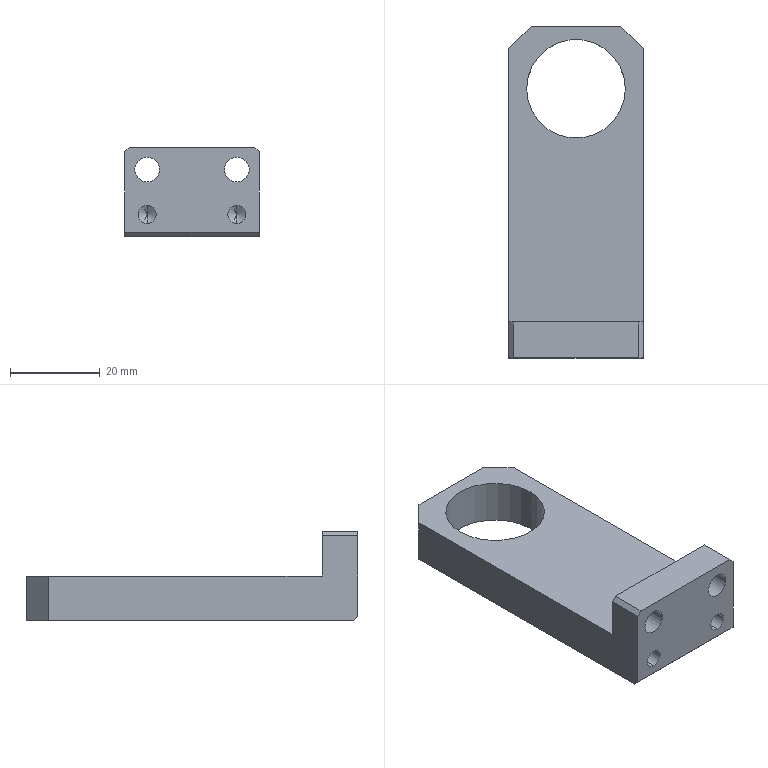Part | SolidWorks | features Chamfer 2, ICE 2, Extrusion 1, HoleWzd 1 | 1 solid | 27 faces | box 30 x 74 x 20 mm | volume 19884 mm3 | plane 13 | cylinder 10 | cone 4 | commonest cylinder face diameters 4 x4 5.5 x4 22 x2
STEP:
#1=CARTESIAN_POINT('',(-10.,10.,7.));
#2=VERTEX_POINT('',#1);
#3=CARTESIAN_POINT('',(-10.,10.,3.));
#4=VERTEX_POINT('',#3);
#5=CARTESIAN_POINT('',(-10.,10.,5.));
#6=DIRECTION('',(0.,-1.,0.));
#7=DIRECTION('',(0.,0.,-1.));
#8=AXIS2_PLACEMENT_3D('',#5,#6,#7);
#9=CIRCLE('',#8,2.);
#10=EDGE_CURVE('',#2,#4,#9,.T.);
#11=ORIENTED_EDGE('',*,*,#10,.F.);
#12=CARTESIAN_POINT('',(-10.,0.,7.));
#13=VERTEX_POINT('',#12);
#14=CARTESIAN_POINT('',(-10.,0.,7.));
#15=DIRECTION('',(0.,-1.,0.));
#16=VECTOR('',#15,1000.);
#17=LINE('',#14,#16);
#18=EDGE_CURVE('',#2,#13,#17,.T.);
#19=ORIENTED_EDGE('',*,*,#18,.T.);
#20=CARTESIAN_POINT('',(-10.,0.,3.));
#21=VERTEX_POINT('',#20);
#22=CARTESIAN_POINT('',(-10.,0.,5.));
#23=DIRECTION('',(0.,-1.,0.));
#24=DIRECTION('',(0.,0.,-1.));
#25=AXIS2_PLACEMENT_3D('',#22,#23,#24);
#26=CIRCLE('',#25,2.);
#27=EDGE_CURVE('',#13,#21,#26,.T.);
#28=ORIENTED_EDGE('',*,*,#27,.T.);
#29=CARTESIAN_POINT('',(-10.,0.,3.));
#30=DIRECTION('',(0.,-1.,0.));
#31=VECTOR('',#30,1000.);
#32=LINE('',#29,#31);
#33=EDGE_CURVE('',#4,#21,#32,.T.);
#34=ORIENTED_EDGE('',*,*,#33,.F.);
#35=EDGE_LOOP('',(#11,#19,#28,#34));
#36=FACE_OUTER_BOUND('',#35,.T.);
#37=CARTESIAN_POINT('',(-10.,0.,5.));
#38=DIRECTION('',(0.,-1.,0.));
#39=DIRECTION('',(0.,0.,-1.));
#40=AXIS2_PLACEMENT_3D('',#37,#38,#39);
#41=CYLINDRICAL_SURFACE('',#40,2.);
#42=ADVANCED_FACE('',(#36),#41,.F.);
#43=CARTESIAN_POINT('',(-10.,11.202,5.));
#44=VERTEX_POINT('',#43);
#45=CARTESIAN_POINT('',(-10.,10.,3.));
#46=DIRECTION('',(0.,-0.515,-0.8572));
#47=VECTOR('',#46,1000.);
#48=LINE('',#45,#47);
#49=EDGE_CURVE('',#44,#4,#48,.T.);
#50=ORIENTED_EDGE('',*,*,#49,.F.);
#51=CARTESIAN_POINT('',(-10.,10.,7.));
#52=DIRECTION('',(0.,-0.515,0.8572));
#53=VECTOR('',#52,1000.);
#54=LINE('',#51,#53);
#55=EDGE_CURVE('',#44,#2,#54,.T.);
#56=ORIENTED_EDGE('',*,*,#55,.T.);
#57=ORIENTED_EDGE('',*,*,#10,.T.);
#58=EDGE_LOOP('',(#50,#56,#57));
#59=FACE_OUTER_BOUND('',#58,.T.);
#60=CARTESIAN_POINT('',(-10.,10.,5.));
#61=DIRECTION('',(0.,-1.,0.));
#62=DIRECTION('',(0.,0.,-1.));
#63=AXIS2_PLACEMENT_3D('',#60,#61,#62);
#64=CONICAL_SURFACE('',#63,2.,1.03);
#65=ADVANCED_FACE('',(#59),#64,.F.);
#66=CARTESIAN_POINT('',(10.,10.,7.));
#67=VERTEX_POINT('',#66);
#68=CARTESIAN_POINT('',(10.,10.,3.));
#69=VERTEX_POINT('',#68);
#70=CARTESIAN_POINT('',(10.,10.,5.));
#71=DIRECTION('',(0.,-1.,0.));
#72=DIRECTION('',(0.,0.,-1.));
#73=AXIS2_PLACEMENT_3D('',#70,#71,#72);
#74=CIRCLE('',#73,2.);
#75=EDGE_CURVE('',#67,#69,#74,.T.);
#76=ORIENTED_EDGE('',*,*,#75,.F.);
#77=CARTESIAN_POINT('',(10.,0.,7.));
#78=VERTEX_POINT('',#77);
#79=CARTESIAN_POINT('',(10.,0.,7.));
#80=DIRECTION('',(0.,-1.,0.));
#81=VECTOR('',#80,1000.);
#82=LINE('',#79,#81);
#83=EDGE_CURVE('',#67,#78,#82,.T.);
#84=ORIENTED_EDGE('',*,*,#83,.T.);
#85=CARTESIAN_POINT('',(10.,0.,3.));
#86=VERTEX_POINT('',#85);
#87=CARTESIAN_POINT('',(10.,0.,5.));
#88=DIRECTION('',(0.,-1.,0.));
#89=DIRECTION('',(0.,0.,-1.));
#90=AXIS2_PLACEMENT_3D('',#87,#88,#89);
#91=CIRCLE('',#90,2.);
#92=EDGE_CURVE('',#78,#86,#91,.T.);
#93=ORIENTED_EDGE('',*,*,#92,.T.);
#94=CARTESIAN_POINT('',(10.,0.,3.));
#95=DIRECTION('',(0.,-1.,0.));
#96=VECTOR('',#95,1000.);
#97=LINE('',#94,#96);
#98=EDGE_CURVE('',#69,#86,#97,.T.);
#99=ORIENTED_EDGE('',*,*,#98,.F.);
#100=EDGE_LOOP('',(#76,#84,#93,#99));
#101=FACE_OUTER_BOUND('',#100,.T.);
#102=CARTESIAN_POINT('',(10.,0.,5.));
#103=DIRECTION('',(0.,-1.,0.));
#104=DIRECTION('',(0.,0.,-1.));
#105=AXIS2_PLACEMENT_3D('',#102,#103,#104);
#106=CYLINDRICAL_SURFACE('',#105,2.);
#107=ADVANCED_FACE('',(#101),#106,.F.);
#108=CARTESIAN_POINT('',(10.,11.202,5.));
#109=VERTEX_POINT('',#108);
#110=CARTESIAN_POINT('',(10.,10.,3.));
#111=DIRECTION('',(0.,-0.515,-0.8572));
#112=VECTOR('',#111,1000.);
#113=LINE('',#110,#112);
#114=EDGE_CURVE('',#109,#69,#113,.T.);
#115=ORIENTED_EDGE('',*,*,#114,.F.);
#116=CARTESIAN_POINT('',(10.,10.,7.));
#117=DIRECTION('',(0.,-0.515,0.8572));
#118=VECTOR('',#117,1000.);
#119=LINE('',#116,#118);
#120=EDGE_CURVE('',#109,#67,#119,.T.);
#121=ORIENTED_EDGE('',*,*,#120,.T.);
#122=ORIENTED_EDGE('',*,*,#75,.T.);
#123=EDGE_LOOP('',(#115,#121,#122));
#124=FACE_OUTER_BOUND('',#123,.T.);
#125=CARTESIAN_POINT('',(10.,10.,5.));
#126=DIRECTION('',(0.,-1.,0.));
#127=DIRECTION('',(0.,0.,-1.));
#128=AXIS2_PLACEMENT_3D('',#125,#126,#127);
#129=CONICAL_SURFACE('',#128,2.,1.03);
#130=ADVANCED_FACE('',(#124),#129,.F.);
#131=CARTESIAN_POINT('',(12.75,0.,15.));
#132=VERTEX_POINT('',#131);
#133=CARTESIAN_POINT('',(7.25,0.,15.));
#134=VERTEX_POINT('',#133);
#135=CARTESIAN_POINT('',(10.,0.,15.));
#136=DIRECTION('',(0.,1.,0.));
#137=DIRECTION('',(1.,0.,0.));
#138=AXIS2_PLACEMENT_3D('',#135,#136,#137);
#139=CIRCLE('',#138,2.75);
#140=EDGE_CURVE('',#132,#134,#139,.T.);
#141=ORIENTED_EDGE('',*,*,#140,.F.);
#142=CARTESIAN_POINT('',(12.75,8.,15.));
#143=VERTEX_POINT('',#142);
#144=CARTESIAN_POINT('',(12.75,0.,15.));
#145=DIRECTION('',(0.,1.,0.));
#146=VECTOR('',#145,1000.);
#147=LINE('',#144,#146);
#148=EDGE_CURVE('',#132,#143,#147,.T.);
#149=ORIENTED_EDGE('',*,*,#148,.T.);
#150=CARTESIAN_POINT('',(7.25,8.,15.));
#151=VERTEX_POINT('',#150);
#152=CARTESIAN_POINT('',(10.,8.,15.));
#153=DIRECTION('',(0.,1.,0.));
#154=DIRECTION('',(1.,0.,0.));
#155=AXIS2_PLACEMENT_3D('',#152,#153,#154);
#156=CIRCLE('',#155,2.75);
#157=EDGE_CURVE('',#143,#151,#156,.T.);
#158=ORIENTED_EDGE('',*,*,#157,.T.);
#159=CARTESIAN_POINT('',(7.25,0.,15.));
#160=DIRECTION('',(0.,1.,0.));
#161=VECTOR('',#160,1000.);
#162=LINE('',#159,#161);
#163=EDGE_CURVE('',#134,#151,#162,.T.);
#164=ORIENTED_EDGE('',*,*,#163,.F.);
#165=EDGE_LOOP('',(#141,#149,#158,#164));
#166=FACE_OUTER_BOUND('',#165,.T.);
#167=CARTESIAN_POINT('',(10.,0.,15.));
#168=DIRECTION('',(0.,1.,0.));
#169=DIRECTION('',(-1.,0.,0.));
#170=AXIS2_PLACEMENT_3D('',#167,#168,#169);
#171=CYLINDRICAL_SURFACE('',#170,2.75);
#172=ADVANCED_FACE('',(#166),#171,.F.);
#173=CARTESIAN_POINT('',(-7.25,0.,15.));
#174=VERTEX_POINT('',#173);
#175=CARTESIAN_POINT('',(-12.75,0.,15.));
#176=VERTEX_POINT('',#175);
#177=CARTESIAN_POINT('',(-10.,0.,15.));
#178=DIRECTION('',(0.,1.,0.));
#179=DIRECTION('',(-1.,0.,0.));
#180=AXIS2_PLACEMENT_3D('',#177,#178,#179);
#181=CIRCLE('',#180,2.75);
#182=EDGE_CURVE('',#174,#176,#181,.T.);
#183=ORIENTED_EDGE('',*,*,#182,.F.);
#184=CARTESIAN_POINT('',(-7.25,8.,15.));
#185=VERTEX_POINT('',#184);
#186=CARTESIAN_POINT('',(-7.25,0.,15.));
#187=DIRECTION('',(0.,1.,0.));
#188=VECTOR('',#187,1000.);
#189=LINE('',#186,#188);
#190=EDGE_CURVE('',#174,#185,#189,.T.);
#191=ORIENTED_EDGE('',*,*,#190,.T.);
#192=CARTESIAN_POINT('',(-12.75,8.,15.));
#193=VERTEX_POINT('',#192);
#194=CARTESIAN_POINT('',(-10.,8.,15.));
#195=DIRECTION('',(0.,1.,0.));
#196=DIRECTION('',(-1.,0.,0.));
#197=AXIS2_PLACEMENT_3D('',#194,#195,#196);
#198=CIRCLE('',#197,2.75);
#199=EDGE_CURVE('',#185,#193,#198,.T.);
#200=ORIENTED_EDGE('',*,*,#199,.T.);
#201=CARTESIAN_POINT('',(-12.75,0.,15.));
#202=DIRECTION('',(0.,1.,0.));
#203=VECTOR('',#202,1000.);
#204=LINE('',#201,#203);
#205=EDGE_CURVE('',#176,#193,#204,.T.);
#206=ORIENTED_EDGE('',*,*,#205,.F.);
#207=EDGE_LOOP('',(#183,#191,#200,#206));
#208=FACE_OUTER_BOUND('',#207,.T.);
#209=CARTESIAN_POINT('',(-10.,0.,15.));
#210=DIRECTION('',(0.,1.,0.));
#211=DIRECTION('',(-1.,0.,0.));
#212=AXIS2_PLACEMENT_3D('',#209,#210,#211);
#213=CYLINDRICAL_SURFACE('',#212,2.75);
#214=ADVANCED_FACE('',(#208),#213,.F.);
#215=CARTESIAN_POINT('',(-11.,60.,10.));
#216=VERTEX_POINT('',#215);
#217=CARTESIAN_POINT('',(11.,60.,10.));
#218=VERTEX_POINT('',#217);
#219=CARTESIAN_POINT('',(0.,60.,10.));
#220=DIRECTION('',(0.,0.,1.));
#221=DIRECTION('',(1.,0.,0.));
#222=AXIS2_PLACEMENT_3D('',#219,#220,#221);
#223=CIRCLE('',#222,11.);
#224=EDGE_CURVE('',#216,#218,#223,.T.);
#225=ORIENTED_EDGE('',*,*,#224,.T.);
#226=CARTESIAN_POINT('',(11.,60.,0.));
#227=VERTEX_POINT('',#226);
#228=CARTESIAN_POINT('',(11.,60.,10.));
#229=DIRECTION('',(0.,0.,-1.));
#230=VECTOR('',#229,1000.);
#231=LINE('',#228,#230);
#232=EDGE_CURVE('',#218,#227,#231,.T.);
#233=ORIENTED_EDGE('',*,*,#232,.T.);
#234=CARTESIAN_POINT('',(-11.,60.,0.));
#235=VERTEX_POINT('',#234);
#236=CARTESIAN_POINT('',(0.,60.,0.));
#237=DIRECTION('',(0.,0.,1.));
#238=DIRECTION('',(1.,0.,0.));
#239=AXIS2_PLACEMENT_3D('',#236,#237,#238);
#240=CIRCLE('',#239,11.);
#241=EDGE_CURVE('',#235,#227,#240,.T.);
#242=ORIENTED_EDGE('',*,*,#241,.F.);
#243=CARTESIAN_POINT('',(-11.,60.,10.));
#244=DIRECTION('',(0.,0.,-1.));
#245=VECTOR('',#244,1000.);
#246=LINE('',#243,#245);
#247=EDGE_CURVE('',#216,#235,#246,.T.);
#248=ORIENTED_EDGE('',*,*,#247,.F.);
#249=EDGE_LOOP('',(#225,#233,#242,#248));
#250=FACE_OUTER_BOUND('',#249,.T.);
#251=CARTESIAN_POINT('',(0.,60.,10.));
#252=DIRECTION('',(0.,0.,-1.));
#253=DIRECTION('',(-1.,0.,0.));
#254=AXIS2_PLACEMENT_3D('',#251,#252,#253);
#255=CYLINDRICAL_SURFACE('',#254,11.);
#256=ADVANCED_FACE('',(#250),#255,.F.);
#257=CARTESIAN_POINT('',(10.,74.,10.));
#258=VERTEX_POINT('',#257);
#259=CARTESIAN_POINT('',(-10.,74.,10.));
#260=VERTEX_POINT('',#259);
#261=CARTESIAN_POINT('',(15.,74.,10.));
#262=DIRECTION('',(-1.,0.,0.));
#263=VECTOR('',#262,1000.);
#264=LINE('',#261,#263);
#265=EDGE_CURVE('',#258,#260,#264,.T.);
#266=ORIENTED_EDGE('',*,*,#265,.T.);
#267=CARTESIAN_POINT('',(-15.,69.,10.));
#268=VERTEX_POINT('',#267);
#269=CARTESIAN_POINT('',(-12.5,71.5,10.));
#270=DIRECTION('',(-0.7071,-0.7071,0.));
#271=VECTOR('',#270,1000.);
#272=LINE('',#269,#271);
#273=EDGE_CURVE('',#260,#268,#272,.T.);
#274=ORIENTED_EDGE('',*,*,#273,.T.);
#275=CARTESIAN_POINT('',(-15.,8.,10.));
#276=VERTEX_POINT('',#275);
#277=CARTESIAN_POINT('',(-15.,0.,10.));
#278=DIRECTION('',(0.,-1.,0.));
#279=VECTOR('',#278,1000.);
#280=LINE('',#277,#279);
#281=EDGE_CURVE('',#268,#276,#280,.T.);
#282=ORIENTED_EDGE('',*,*,#281,.T.);
#283=CARTESIAN_POINT('',(15.,8.,10.));
#284=VERTEX_POINT('',#283);
#285=CARTESIAN_POINT('',(0.,8.,10.));
#286=DIRECTION('',(-1.,0.,0.));
#287=VECTOR('',#286,1000.);
#288=LINE('',#285,#287);
#289=EDGE_CURVE('',#284,#276,#288,.T.);
#290=ORIENTED_EDGE('',*,*,#289,.F.);
#291=CARTESIAN_POINT('',(15.,69.,10.));
#292=VERTEX_POINT('',#291);
#293=CARTESIAN_POINT('',(15.,0.,10.));
#294=DIRECTION('',(0.,1.,0.));
#295=VECTOR('',#294,1000.);
#296=LINE('',#293,#295);
#297=EDGE_CURVE('',#284,#292,#296,.T.);
#298=ORIENTED_EDGE('',*,*,#297,.T.);
#299=CARTESIAN_POINT('',(-2.5,86.5,10.));
#300=DIRECTION('',(-0.7071,0.7071,0.));
#301=VECTOR('',#300,1000.);
#302=LINE('',#299,#301);
#303=EDGE_CURVE('',#292,#258,#302,.T.);
#304=ORIENTED_EDGE('',*,*,#303,.T.);
#305=EDGE_LOOP('',(#266,#274,#282,#290,#298,#304));
#306=FACE_OUTER_BOUND('',#305,.T.);
#307=ORIENTED_EDGE('',*,*,#224,.F.);
#308=CARTESIAN_POINT('',(0.,60.,10.));
#309=DIRECTION('',(0.,0.,1.));
#310=DIRECTION('',(1.,0.,0.));
#311=AXIS2_PLACEMENT_3D('',#308,#309,#310);
#312=CIRCLE('',#311,11.);
#313=EDGE_CURVE('',#218,#216,#312,.T.);
#314=ORIENTED_EDGE('',*,*,#313,.F.);
#315=EDGE_LOOP('',(#307,#314));
#316=FACE_BOUND('',#315,.T.);
#317=CARTESIAN_POINT('',(-15.,74.,10.));
#318=DIRECTION('',(0.,0.,1.));
#319=DIRECTION('',(1.,0.,0.));
#320=AXIS2_PLACEMENT_3D('',#317,#318,#319);
#321=PLANE('',#320);
#322=ADVANCED_FACE('',(#306,#316),#321,.T.);
#323=CARTESIAN_POINT('',(15.,1.,0.));
#324=VERTEX_POINT('',#323);
#325=CARTESIAN_POINT('',(15.,69.,0.));
#326=VERTEX_POINT('',#325);
#327=CARTESIAN_POINT('',(15.,0.,0.));
#328=DIRECTION('',(0.,1.,0.));
#329=VECTOR('',#328,1000.);
#330=LINE('',#327,#329);
#331=EDGE_CURVE('',#324,#326,#330,.T.);
#332=ORIENTED_EDGE('',*,*,#331,.F.);
#333=CARTESIAN_POINT('',(-15.,1.,0.));
#334=VERTEX_POINT('',#333);
#335=CARTESIAN_POINT('',(-15.,1.,0.));
#336=DIRECTION('',(-1.,0.,0.));
#337=VECTOR('',#336,1000.);
#338=LINE('',#335,#337);
#339=EDGE_CURVE('',#324,#334,#338,.T.);
#340=ORIENTED_EDGE('',*,*,#339,.T.);
#341=CARTESIAN_POINT('',(-15.,69.,0.));
#342=VERTEX_POINT('',#341);
#343=CARTESIAN_POINT('',(-15.,0.,0.));
#344=DIRECTION('',(0.,-1.,0.));
#345=VECTOR('',#344,1000.);
#346=LINE('',#343,#345);
#347=EDGE_CURVE('',#342,#334,#346,.T.);
#348=ORIENTED_EDGE('',*,*,#347,.F.);
#349=CARTESIAN_POINT('',(-10.,74.,0.));
#350=VERTEX_POINT('',#349);
#351=CARTESIAN_POINT('',(-15.,69.,0.));
#352=DIRECTION('',(0.7071,0.7071,0.));
#353=VECTOR('',#352,1000.);
#354=LINE('',#351,#353);
#355=EDGE_CURVE('',#342,#350,#354,.T.);
#356=ORIENTED_EDGE('',*,*,#355,.T.);
#357=CARTESIAN_POINT('',(10.,74.,0.));
#358=VERTEX_POINT('',#357);
#359=CARTESIAN_POINT('',(15.,74.,0.));
#360=DIRECTION('',(-1.,0.,0.));
#361=VECTOR('',#360,1000.);
#362=LINE('',#359,#361);
#363=EDGE_CURVE('',#358,#350,#362,.T.);
#364=ORIENTED_EDGE('',*,*,#363,.F.);
#365=CARTESIAN_POINT('',(10.,74.,0.));
#366=DIRECTION('',(0.7071,-0.7071,0.));
#367=VECTOR('',#366,1000.);
#368=LINE('',#365,#367);
#369=EDGE_CURVE('',#358,#326,#368,.T.);
#370=ORIENTED_EDGE('',*,*,#369,.T.);
#371=EDGE_LOOP('',(#332,#340,#348,#356,#364,#370));
#372=FACE_OUTER_BOUND('',#371,.T.);
#373=ORIENTED_EDGE('',*,*,#241,.T.);
#374=CARTESIAN_POINT('',(0.,60.,0.));
#375=DIRECTION('',(0.,0.,1.));
#376=DIRECTION('',(1.,0.,0.));
#377=AXIS2_PLACEMENT_3D('',#374,#375,#376);
#378=CIRCLE('',#377,11.);
#379=EDGE_CURVE('',#227,#235,#378,.T.);
#380=ORIENTED_EDGE('',*,*,#379,.T.);
#381=EDGE_LOOP('',(#373,#380));
#382=FACE_BOUND('',#381,.T.);
#383=CARTESIAN_POINT('',(-15.,74.,0.));
#384=DIRECTION('',(0.,0.,1.));
#385=DIRECTION('',(1.,0.,0.));
#386=AXIS2_PLACEMENT_3D('',#383,#384,#385);
#387=PLANE('',#386);
#388=ADVANCED_FACE('',(#372,#382),#387,.F.);
#389=ORIENTED_EDGE('',*,*,#347,.T.);
#390=CARTESIAN_POINT('',(-15.,0.,1.));
#391=VERTEX_POINT('',#390);
#392=CARTESIAN_POINT('',(-15.,0.,1.));
#393=DIRECTION('',(0.,-0.7071,0.7071));
#394=VECTOR('',#393,1000.);
#395=LINE('',#392,#394);
#396=EDGE_CURVE('',#334,#391,#395,.T.);
#397=ORIENTED_EDGE('',*,*,#396,.T.);
#398=CARTESIAN_POINT('',(-15.,0.,19.));
#399=VERTEX_POINT('',#398);
#400=CARTESIAN_POINT('',(-15.,0.,10.));
#401=DIRECTION('',(0.,0.,-1.));
#402=VECTOR('',#401,1000.);
#403=LINE('',#400,#402);
#404=EDGE_CURVE('',#399,#391,#403,.T.);
#405=ORIENTED_EDGE('',*,*,#404,.F.);
#406=CARTESIAN_POINT('',(-15.,8.,19.));
#407=VERTEX_POINT('',#406);
#408=CARTESIAN_POINT('',(-15.,0.,19.));
#409=DIRECTION('',(0.,1.,0.));
#410=VECTOR('',#409,1000.);
#411=LINE('',#408,#410);
#412=EDGE_CURVE('',#399,#407,#411,.T.);
#413=ORIENTED_EDGE('',*,*,#412,.T.);
#414=CARTESIAN_POINT('',(-15.,8.,0.));
#415=DIRECTION('',(0.,0.,1.));
#416=VECTOR('',#415,1000.);
#417=LINE('',#414,#416);
#418=EDGE_CURVE('',#276,#407,#417,.T.);
#419=ORIENTED_EDGE('',*,*,#418,.F.);
#420=ORIENTED_EDGE('',*,*,#281,.F.);
#421=CARTESIAN_POINT('',(-15.,69.,10.));
#422=DIRECTION('',(0.,0.,-1.));
#423=VECTOR('',#422,1000.);
#424=LINE('',#421,#423);
#425=EDGE_CURVE('',#268,#342,#424,.T.);
#426=ORIENTED_EDGE('',*,*,#425,.T.);
#427=EDGE_LOOP('',(#389,#397,#405,#413,#419,#420,#426));
#428=FACE_OUTER_BOUND('',#427,.T.);
#429=CARTESIAN_POINT('',(-15.,0.,10.));
#430=DIRECTION('',(1.,0.,0.));
#431=DIRECTION('',(0.,0.,-1.));
#432=AXIS2_PLACEMENT_3D('',#429,#430,#431);
#433=PLANE('',#432);
#434=ADVANCED_FACE('',(#428),#433,.F.);
#435=CARTESIAN_POINT('',(-10.,0.,5.));
#436=DIRECTION('',(0.,-1.,0.));
#437=DIRECTION('',(0.,0.,-1.));
#438=AXIS2_PLACEMENT_3D('',#435,#436,#437);
#439=CIRCLE('',#438,2.);
#440=EDGE_CURVE('',#21,#13,#439,.T.);
#441=ORIENTED_EDGE('',*,*,#440,.F.);
#442=ORIENTED_EDGE('',*,*,#27,.F.);
#443=EDGE_LOOP('',(#441,#442));
#444=FACE_BOUND('',#443,.T.);
#445=CARTESIAN_POINT('',(10.,0.,5.));
#446=DIRECTION('',(0.,-1.,0.));
#447=DIRECTION('',(0.,0.,-1.));
#448=AXIS2_PLACEMENT_3D('',#445,#446,#447);
#449=CIRCLE('',#448,2.);
#450=EDGE_CURVE('',#86,#78,#449,.T.);
#451=ORIENTED_EDGE('',*,*,#450,.F.);
#452=ORIENTED_EDGE('',*,*,#92,.F.);
#453=EDGE_LOOP('',(#451,#452));
#454=FACE_BOUND('',#453,.T.);
#455=CARTESIAN_POINT('',(10.,0.,15.));
#456=DIRECTION('',(0.,1.,0.));
#457=DIRECTION('',(1.,0.,0.));
#458=AXIS2_PLACEMENT_3D('',#455,#456,#457);
#459=CIRCLE('',#458,2.75);
#460=EDGE_CURVE('',#134,#132,#459,.T.);
#461=ORIENTED_EDGE('',*,*,#460,.T.);
#462=ORIENTED_EDGE('',*,*,#140,.T.);
#463=EDGE_LOOP('',(#461,#462));
#464=FACE_BOUND('',#463,.T.);
#465=CARTESIAN_POINT('',(-10.,0.,15.));
#466=DIRECTION('',(0.,1.,0.));
#467=DIRECTION('',(-1.,0.,0.));
#468=AXIS2_PLACEMENT_3D('',#465,#466,#467);
#469=CIRCLE('',#468,2.75);
#470=EDGE_CURVE('',#176,#174,#469,.T.);
#471=ORIENTED_EDGE('',*,*,#470,.T.);
#472=ORIENTED_EDGE('',*,*,#182,.T.);
#473=EDGE_LOOP('',(#471,#472));
#474=FACE_BOUND('',#473,.T.);
#475=ORIENTED_EDGE('',*,*,#404,.T.);
#476=CARTESIAN_POINT('',(15.,0.,1.));
#477=VERTEX_POINT('',#476);
#478=CARTESIAN_POINT('',(15.,0.,1.));
#479=DIRECTION('',(1.,0.,0.));
#480=VECTOR('',#479,1000.);
#481=LINE('',#478,#480);
#482=EDGE_CURVE('',#391,#477,#481,.T.);
#483=ORIENTED_EDGE('',*,*,#482,.T.);
#484=CARTESIAN_POINT('',(15.,0.,19.));
#485=VERTEX_POINT('',#484);
#486=CARTESIAN_POINT('',(15.,0.,10.));
#487=DIRECTION('',(0.,0.,-1.));
#488=VECTOR('',#487,1000.);
#489=LINE('',#486,#488);
#490=EDGE_CURVE('',#485,#477,#489,.T.);
#491=ORIENTED_EDGE('',*,*,#490,.F.);
#492=CARTESIAN_POINT('',(14.,0.,20.));
#493=VERTEX_POINT('',#492);
#494=CARTESIAN_POINT('',(15.,0.,19.));
#495=DIRECTION('',(-0.7071,0.,0.7071));
#496=VECTOR('',#495,1000.);
#497=LINE('',#494,#496);
#498=EDGE_CURVE('',#485,#493,#497,.T.);
#499=ORIENTED_EDGE('',*,*,#498,.T.);
#500=CARTESIAN_POINT('',(-14.,0.,20.));
#501=VERTEX_POINT('',#500);
#502=CARTESIAN_POINT('',(0.,0.,20.));
#503=DIRECTION('',(1.,0.,0.));
#504=VECTOR('',#503,1000.);
#505=LINE('',#502,#504);
#506=EDGE_CURVE('',#501,#493,#505,.T.);
#507=ORIENTED_EDGE('',*,*,#506,.F.);
#508=CARTESIAN_POINT('',(-14.,0.,20.));
#509=DIRECTION('',(-0.7071,0.,-0.7071));
#510=VECTOR('',#509,1000.);
#511=LINE('',#508,#510);
#512=EDGE_CURVE('',#501,#399,#511,.T.);
#513=ORIENTED_EDGE('',*,*,#512,.T.);
#514=EDGE_LOOP('',(#475,#483,#491,#499,#507,#513));
#515=FACE_OUTER_BOUND('',#514,.T.);
#516=CARTESIAN_POINT('',(15.,0.,10.));
#517=DIRECTION('',(0.,1.,0.));
#518=DIRECTION('',(0.,0.,1.));
#519=AXIS2_PLACEMENT_3D('',#516,#517,#518);
#520=PLANE('',#519);
#521=ADVANCED_FACE('',(#444,#454,#464,#474,#515),#520,.F.);
#522=ORIENTED_EDGE('',*,*,#490,.T.);
#523=CARTESIAN_POINT('',(15.,0.,1.));
#524=DIRECTION('',(0.,0.7071,-0.7071));
#525=VECTOR('',#524,1000.);
#526=LINE('',#523,#525);
#527=EDGE_CURVE('',#477,#324,#526,.T.);
#528=ORIENTED_EDGE('',*,*,#527,.T.);
#529=ORIENTED_EDGE('',*,*,#331,.T.);
#530=CARTESIAN_POINT('',(15.,69.,10.));
#531=DIRECTION('',(0.,0.,1.));
#532=VECTOR('',#531,1000.);
#533=LINE('',#530,#532);
#534=EDGE_CURVE('',#326,#292,#533,.T.);
#535=ORIENTED_EDGE('',*,*,#534,.T.);
#536=ORIENTED_EDGE('',*,*,#297,.F.);
#537=CARTESIAN_POINT('',(15.,8.,19.));
#538=VERTEX_POINT('',#537);
#539=CARTESIAN_POINT('',(15.,8.,0.));
#540=DIRECTION('',(0.,0.,1.));
#541=VECTOR('',#540,1000.);
#542=LINE('',#539,#541);
#543=EDGE_CURVE('',#284,#538,#542,.T.);
#544=ORIENTED_EDGE('',*,*,#543,.T.);
#545=CARTESIAN_POINT('',(15.,0.,19.));
#546=DIRECTION('',(0.,-1.,0.));
#547=VECTOR('',#546,1000.);
#548=LINE('',#545,#547);
#549=EDGE_CURVE('',#538,#485,#548,.T.);
#550=ORIENTED_EDGE('',*,*,#549,.T.);
#551=EDGE_LOOP('',(#522,#528,#529,#535,#536,#544,#550));
#552=FACE_OUTER_BOUND('',#551,.T.);
#553=CARTESIAN_POINT('',(15.,0.,10.));
#554=DIRECTION('',(-1.,0.,0.));
#555=DIRECTION('',(0.,0.,1.));
#556=AXIS2_PLACEMENT_3D('',#553,#554,#555);
#557=PLANE('',#556);
#558=ADVANCED_FACE('',(#552),#557,.F.);
#559=ORIENTED_EDGE('',*,*,#363,.T.);
#560=CARTESIAN_POINT('',(-10.,74.,10.));
#561=DIRECTION('',(0.,0.,1.));
#562=VECTOR('',#561,1000.);
#563=LINE('',#560,#562);
#564=EDGE_CURVE('',#350,#260,#563,.T.);
#565=ORIENTED_EDGE('',*,*,#564,.T.);
#566=ORIENTED_EDGE('',*,*,#265,.F.);
#567=CARTESIAN_POINT('',(10.,74.,10.));
#568=DIRECTION('',(0.,0.,-1.));
#569=VECTOR('',#568,1000.);
#570=LINE('',#567,#569);
#571=EDGE_CURVE('',#258,#358,#570,.T.);
#572=ORIENTED_EDGE('',*,*,#571,.T.);
#573=EDGE_LOOP('',(#559,#565,#566,#572));
#574=FACE_OUTER_BOUND('',#573,.T.);
#575=CARTESIAN_POINT('',(15.,74.,10.));
#576=DIRECTION('',(0.,-1.,0.));
#577=DIRECTION('',(0.,0.,-1.));
#578=AXIS2_PLACEMENT_3D('',#575,#576,#577);
#579=PLANE('',#578);
#580=ADVANCED_FACE('',(#574),#579,.F.);
#581=ORIENTED_EDGE('',*,*,#232,.F.);
#582=ORIENTED_EDGE('',*,*,#313,.T.);
#583=ORIENTED_EDGE('',*,*,#247,.T.);
#584=ORIENTED_EDGE('',*,*,#379,.F.);
#585=EDGE_LOOP('',(#581,#582,#583,#584));
#586=FACE_OUTER_BOUND('',#585,.T.);
#587=CARTESIAN_POINT('',(0.,60.,10.));
#588=DIRECTION('',(0.,0.,-1.));
#589=DIRECTION('',(-1.,0.,0.));
#590=AXIS2_PLACEMENT_3D('',#587,#588,#589);
#591=CYLINDRICAL_SURFACE('',#590,11.);
#592=ADVANCED_FACE('',(#586),#591,.F.);
#593=CARTESIAN_POINT('',(-14.,8.,20.));
#594=VERTEX_POINT('',#593);
#595=CARTESIAN_POINT('',(14.,8.,20.));
#596=VERTEX_POINT('',#595);
#597=CARTESIAN_POINT('',(0.,8.,20.));
#598=DIRECTION('',(1.,0.,0.));
#599=VECTOR('',#598,1000.);
#600=LINE('',#597,#599);
#601=EDGE_CURVE('',#594,#596,#600,.T.);
#602=ORIENTED_EDGE('',*,*,#601,.F.);
#603=CARTESIAN_POINT('',(-14.,8.,20.));
#604=DIRECTION('',(0.,-1.,0.));
#605=VECTOR('',#604,1000.);
#606=LINE('',#603,#605);
#607=EDGE_CURVE('',#594,#501,#606,.T.);
#608=ORIENTED_EDGE('',*,*,#607,.T.);
#609=ORIENTED_EDGE('',*,*,#506,.T.);
#610=CARTESIAN_POINT('',(14.,8.,20.));
#611=DIRECTION('',(0.,1.,0.));
#612=VECTOR('',#611,1000.);
#613=LINE('',#610,#612);
#614=EDGE_CURVE('',#493,#596,#613,.T.);
#615=ORIENTED_EDGE('',*,*,#614,.T.);
#616=EDGE_LOOP('',(#602,#608,#609,#615));
#617=FACE_OUTER_BOUND('',#616,.T.);
#618=CARTESIAN_POINT('',(0.,8.,20.));
#619=DIRECTION('',(0.,0.,-1.));
#620=DIRECTION('',(-1.,0.,0.));
#621=AXIS2_PLACEMENT_3D('',#618,#619,#620);
#622=PLANE('',#621);
#623=ADVANCED_FACE('',(#617),#622,.F.);
#624=CARTESIAN_POINT('',(10.,8.,15.));
#625=DIRECTION('',(0.,1.,0.));
#626=DIRECTION('',(1.,0.,0.));
#627=AXIS2_PLACEMENT_3D('',#624,#625,#626);
#628=CIRCLE('',#627,2.75);
#629=EDGE_CURVE('',#151,#143,#628,.T.);
#630=ORIENTED_EDGE('',*,*,#629,.F.);
#631=ORIENTED_EDGE('',*,*,#157,.F.);
#632=EDGE_LOOP('',(#630,#631));
#633=FACE_BOUND('',#632,.T.);
#634=CARTESIAN_POINT('',(-10.,8.,15.));
#635=DIRECTION('',(0.,1.,0.));
#636=DIRECTION('',(-1.,0.,0.));
#637=AXIS2_PLACEMENT_3D('',#634,#635,#636);
#638=CIRCLE('',#637,2.75);
#639=EDGE_CURVE('',#193,#185,#638,.T.);
#640=ORIENTED_EDGE('',*,*,#639,.F.);
#641=ORIENTED_EDGE('',*,*,#199,.F.);
#642=EDGE_LOOP('',(#640,#641));
#643=FACE_BOUND('',#642,.T.);
#644=ORIENTED_EDGE('',*,*,#418,.T.);
#645=CARTESIAN_POINT('',(-14.,8.,20.));
#646=DIRECTION('',(0.7071,0.,0.7071));
#647=VECTOR('',#646,1000.);
#648=LINE('',#645,#647);
#649=EDGE_CURVE('',#407,#594,#648,.T.);
#650=ORIENTED_EDGE('',*,*,#649,.T.);
#651=ORIENTED_EDGE('',*,*,#601,.T.);
#652=CARTESIAN_POINT('',(15.,8.,19.));
#653=DIRECTION('',(0.7071,0.,-0.7071));
#654=VECTOR('',#653,1000.);
#655=LINE('',#652,#654);
#656=EDGE_CURVE('',#596,#538,#655,.T.);
#657=ORIENTED_EDGE('',*,*,#656,.T.);
#658=ORIENTED_EDGE('',*,*,#543,.F.);
#659=ORIENTED_EDGE('',*,*,#289,.T.);
#660=EDGE_LOOP('',(#644,#650,#651,#657,#658,#659));
#661=FACE_OUTER_BOUND('',#660,.T.);
#662=CARTESIAN_POINT('',(0.,8.,0.));
#663=DIRECTION('',(0.,-1.,0.));
#664=DIRECTION('',(1.,0.,0.));
#665=AXIS2_PLACEMENT_3D('',#662,#663,#664);
#666=PLANE('',#665);
#667=ADVANCED_FACE('',(#633,#643,#661),#666,.F.);
#668=ORIENTED_EDGE('',*,*,#190,.F.);
#669=ORIENTED_EDGE('',*,*,#470,.F.);
#670=ORIENTED_EDGE('',*,*,#205,.T.);
#671=ORIENTED_EDGE('',*,*,#639,.T.);
#672=EDGE_LOOP('',(#668,#669,#670,#671));
#673=FACE_OUTER_BOUND('',#672,.T.);
#674=CARTESIAN_POINT('',(-10.,0.,15.));
#675=DIRECTION('',(0.,1.,0.));
#676=DIRECTION('',(-1.,0.,0.));
#677=AXIS2_PLACEMENT_3D('',#674,#675,#676);
#678=CYLINDRICAL_SURFACE('',#677,2.75);
#679=ADVANCED_FACE('',(#673),#678,.F.);
#680=ORIENTED_EDGE('',*,*,#148,.F.);
#681=ORIENTED_EDGE('',*,*,#460,.F.);
#682=ORIENTED_EDGE('',*,*,#163,.T.);
#683=ORIENTED_EDGE('',*,*,#629,.T.);
#684=EDGE_LOOP('',(#680,#681,#682,#683));
#685=FACE_OUTER_BOUND('',#684,.T.);
#686=CARTESIAN_POINT('',(10.,0.,15.));
#687=DIRECTION('',(0.,1.,0.));
#688=DIRECTION('',(-1.,0.,0.));
#689=AXIS2_PLACEMENT_3D('',#686,#687,#688);
#690=CYLINDRICAL_SURFACE('',#689,2.75);
#691=ADVANCED_FACE('',(#685),#690,.F.);
#692=ORIENTED_EDGE('',*,*,#120,.F.);
#693=ORIENTED_EDGE('',*,*,#114,.T.);
#694=CARTESIAN_POINT('',(10.,10.,5.));
#695=DIRECTION('',(0.,-1.,0.));
#696=DIRECTION('',(0.,0.,-1.));
#697=AXIS2_PLACEMENT_3D('',#694,#695,#696);
#698=CIRCLE('',#697,2.);
#699=EDGE_CURVE('',#69,#67,#698,.T.);
#700=ORIENTED_EDGE('',*,*,#699,.T.);
#701=EDGE_LOOP('',(#692,#693,#700));
#702=FACE_OUTER_BOUND('',#701,.T.);
#703=CARTESIAN_POINT('',(10.,10.,5.));
#704=DIRECTION('',(0.,-1.,0.));
#705=DIRECTION('',(0.,0.,-1.));
#706=AXIS2_PLACEMENT_3D('',#703,#704,#705);
#707=CONICAL_SURFACE('',#706,2.,1.03);
#708=ADVANCED_FACE('',(#702),#707,.F.);
#709=ORIENTED_EDGE('',*,*,#83,.F.);
#710=ORIENTED_EDGE('',*,*,#699,.F.);
#711=ORIENTED_EDGE('',*,*,#98,.T.);
#712=ORIENTED_EDGE('',*,*,#450,.T.);
#713=EDGE_LOOP('',(#709,#710,#711,#712));
#714=FACE_OUTER_BOUND('',#713,.T.);
#715=CARTESIAN_POINT('',(10.,0.,5.));
#716=DIRECTION('',(0.,-1.,0.));
#717=DIRECTION('',(0.,0.,-1.));
#718=AXIS2_PLACEMENT_3D('',#715,#716,#717);
#719=CYLINDRICAL_SURFACE('',#718,2.);
#720=ADVANCED_FACE('',(#714),#719,.F.);
#721=ORIENTED_EDGE('',*,*,#55,.F.);
#722=ORIENTED_EDGE('',*,*,#49,.T.);
#723=CARTESIAN_POINT('',(-10.,10.,5.));
#724=DIRECTION('',(0.,-1.,0.));
#725=DIRECTION('',(0.,0.,-1.));
#726=AXIS2_PLACEMENT_3D('',#723,#724,#725);
#727=CIRCLE('',#726,2.);
#728=EDGE_CURVE('',#4,#2,#727,.T.);
#729=ORIENTED_EDGE('',*,*,#728,.T.);
#730=EDGE_LOOP('',(#721,#722,#729));
#731=FACE_OUTER_BOUND('',#730,.T.);
#732=CARTESIAN_POINT('',(-10.,10.,5.));
#733=DIRECTION('',(0.,-1.,0.));
#734=DIRECTION('',(0.,0.,-1.));
#735=AXIS2_PLACEMENT_3D('',#732,#733,#734);
#736=CONICAL_SURFACE('',#735,2.,1.03);
#737=ADVANCED_FACE('',(#731),#736,.F.);
#738=ORIENTED_EDGE('',*,*,#18,.F.);
#739=ORIENTED_EDGE('',*,*,#728,.F.);
#740=ORIENTED_EDGE('',*,*,#33,.T.);
#741=ORIENTED_EDGE('',*,*,#440,.T.);
#742=EDGE_LOOP('',(#738,#739,#740,#741));
#743=FACE_OUTER_BOUND('',#742,.T.);
#744=CARTESIAN_POINT('',(-10.,0.,5.));
#745=DIRECTION('',(0.,-1.,0.));
#746=DIRECTION('',(0.,0.,-1.));
#747=AXIS2_PLACEMENT_3D('',#744,#745,#746);
#748=CYLINDRICAL_SURFACE('',#747,2.);
#749=ADVANCED_FACE('',(#743),#748,.F.);
#750=ORIENTED_EDGE('',*,*,#273,.F.);
#751=ORIENTED_EDGE('',*,*,#564,.F.);
#752=ORIENTED_EDGE('',*,*,#355,.F.);
#753=ORIENTED_EDGE('',*,*,#425,.F.);
#754=EDGE_LOOP('',(#750,#751,#752,#753));
#755=FACE_OUTER_BOUND('',#754,.T.);
#756=CARTESIAN_POINT('',(-15.,69.,10.));
#757=DIRECTION('',(0.7071,-0.7071,0.));
#758=DIRECTION('',(0.7071,0.7071,0.));
#759=AXIS2_PLACEMENT_3D('',#756,#757,#758);
#760=PLANE('',#759);
#761=ADVANCED_FACE('',(#755),#760,.F.);
#762=ORIENTED_EDGE('',*,*,#303,.F.);
#763=ORIENTED_EDGE('',*,*,#534,.F.);
#764=ORIENTED_EDGE('',*,*,#369,.F.);
#765=ORIENTED_EDGE('',*,*,#571,.F.);
#766=EDGE_LOOP('',(#762,#763,#764,#765));
#767=FACE_OUTER_BOUND('',#766,.T.);
#768=CARTESIAN_POINT('',(10.,74.,10.));
#769=DIRECTION('',(-0.7071,-0.7071,0.));
#770=DIRECTION('',(0.7071,-0.7071,0.));
#771=AXIS2_PLACEMENT_3D('',#768,#769,#770);
#772=PLANE('',#771);
#773=ADVANCED_FACE('',(#767),#772,.F.);
#774=ORIENTED_EDGE('',*,*,#396,.F.);
#775=ORIENTED_EDGE('',*,*,#339,.F.);
#776=ORIENTED_EDGE('',*,*,#527,.F.);
#777=ORIENTED_EDGE('',*,*,#482,.F.);
#778=EDGE_LOOP('',(#774,#775,#776,#777));
#779=FACE_OUTER_BOUND('',#778,.T.);
#780=CARTESIAN_POINT('',(15.,0.,1.));
#781=DIRECTION('',(0.,0.7071,0.7071));
#782=DIRECTION('',(0.,-0.7071,0.7071));
#783=AXIS2_PLACEMENT_3D('',#780,#781,#782);
#784=PLANE('',#783);
#785=ADVANCED_FACE('',(#779),#784,.F.);
#786=ORIENTED_EDGE('',*,*,#649,.F.);
#787=ORIENTED_EDGE('',*,*,#412,.F.);
#788=ORIENTED_EDGE('',*,*,#512,.F.);
#789=ORIENTED_EDGE('',*,*,#607,.F.);
#790=EDGE_LOOP('',(#786,#787,#788,#789));
#791=FACE_OUTER_BOUND('',#790,.T.);
#792=CARTESIAN_POINT('',(-14.,8.,20.));
#793=DIRECTION('',(0.7071,0.,-0.7071));
#794=DIRECTION('',(-0.7071,0.,-0.7071));
#795=AXIS2_PLACEMENT_3D('',#792,#793,#794);
#796=PLANE('',#795);
#797=ADVANCED_FACE('',(#791),#796,.F.);
#798=ORIENTED_EDGE('',*,*,#656,.F.);
#799=ORIENTED_EDGE('',*,*,#614,.F.);
#800=ORIENTED_EDGE('',*,*,#498,.F.);
#801=ORIENTED_EDGE('',*,*,#549,.F.);
#802=EDGE_LOOP('',(#798,#799,#800,#801));
#803=FACE_OUTER_BOUND('',#802,.T.);
#804=CARTESIAN_POINT('',(15.,0.,19.));
#805=DIRECTION('',(-0.7071,0.,-0.7071));
#806=DIRECTION('',(-0.7071,0.,0.7071));
#807=AXIS2_PLACEMENT_3D('',#804,#805,#806);
#808=PLANE('',#807);
#809=ADVANCED_FACE('',(#803),#808,.F.);
#810=CLOSED_SHELL('',(#42,#65,#107,#130,#172,#214,#256,#322,#388,#434,#521,#558,#580,#592,#623,#667,#679,#691,#708,#720,#737,#749,#761,#773,#785,#797,#809));
#811=MANIFOLD_SOLID_BREP('',#810);
#812=CARTESIAN_POINT('',(0.,0.,0.));
#813=DIRECTION('',(0.,0.,1.));
#814=DIRECTION('',(1.,0.,0.));
#815=AXIS2_PLACEMENT_3D('',#812,#813,#814);
#816=(LENGTH_UNIT()NAMED_UNIT(*)SI_UNIT(.MILLI.,.METRE.));
#817=UNCERTAINTY_MEASURE_WITH_UNIT(LENGTH_MEASURE(0.00001),#816,'','');
#818=(NAMED_UNIT(*)PLANE_ANGLE_UNIT()SI_UNIT($,.RADIAN.));
#819=(NAMED_UNIT(*)SI_UNIT($,.STERADIAN.)SOLID_ANGLE_UNIT());
#820=(GEOMETRIC_REPRESENTATION_CONTEXT(3)GLOBAL_UNCERTAINTY_ASSIGNED_CONTEXT((#817))GLOBAL_UNIT_ASSIGNED_CONTEXT((#816,#818,#819))REPRESENTATION_CONTEXT('',''));
#821=ADVANCED_BREP_SHAPE_REPRESENTATION('',(#811,#815),#820);